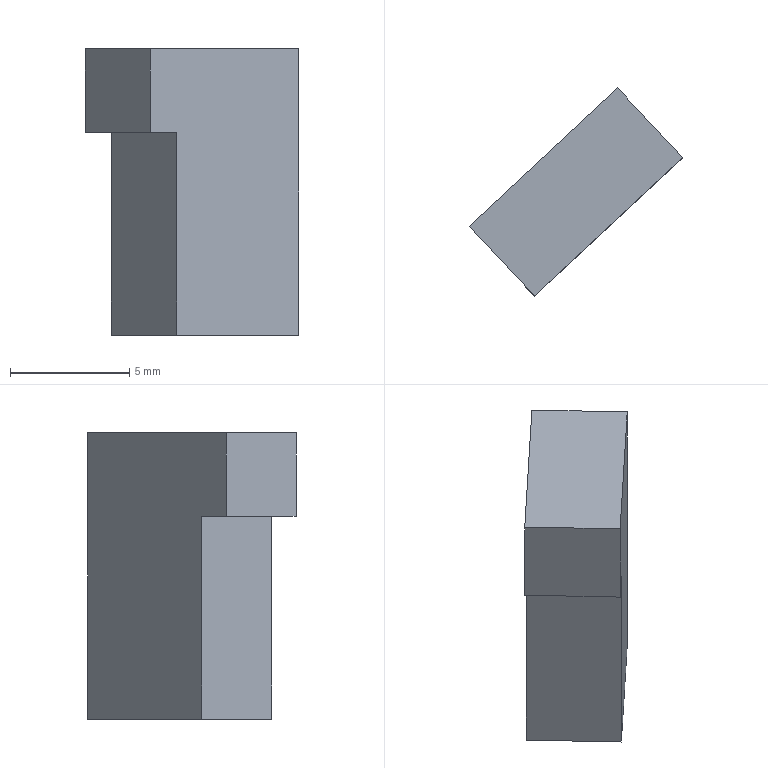Part | STEP file | gslz 2016.10.28-13_id946_x_t | 1 solid | 8 faces | box 8.945 x 8.722 x 12 mm | volume 357 mm3 | plane 8
STEP:
#1=CARTESIAN_POINT('',(0.,0.,0.));
#2=DIRECTION('',(0.,0.,1.));
#3=DIRECTION('',(1.,0.,0.));
#4=AXIS2_PLACEMENT_3D('',#1,#2,#3);
#5=CARTESIAN_POINT('',(-472.551,139.078,1.25));
#6=VERTEX_POINT('',#5);
#7=CARTESIAN_POINT('',(-467.431,143.852,1.25));
#8=VERTEX_POINT('',#7);
#9=CARTESIAN_POINT('',(-472.551,139.078,1.25));
#10=DIRECTION('',(0.7314,0.682,0.));
#11=VECTOR('',#10,1.);
#12=LINE('',#9,#11);
#13=CARTESIAN_POINT('',(-469.961,152.43,1.25));
#14=DIRECTION('',(0.,0.,-1.));
#15=DIRECTION('',(0.7314,0.682,0.));
#16=AXIS2_PLACEMENT_3D('',#13,#14,#15);
#17=PLANE('',#16);
#18=CARTESIAN_POINT('',(-11.,7.999));
#19=DIRECTION('',(1.,0.));
#20=VECTOR('',#19,1.);
#21=LINE('',#18,#20);
#22=(GEOMETRIC_REPRESENTATION_CONTEXT(2)PARAMETRIC_REPRESENTATION_CONTEXT()REPRESENTATION_CONTEXT('',''));
#23=DEFINITIONAL_REPRESENTATION('',(#21),#22);
#24=PCURVE('',#17,#23);
#25=CARTESIAN_POINT('',(-472.551,139.078,-0.75));
#26=DIRECTION('',(0.682,-0.7314,0.));
#27=DIRECTION('',(0.,0.,-1.));
#28=AXIS2_PLACEMENT_3D('',#25,#26,#27);
#29=PLANE('',#28);
#30=CARTESIAN_POINT('',(-2.,0.));
#31=DIRECTION('',(0.,1.));
#32=VECTOR('',#31,1.);
#33=LINE('',#30,#32);
#34=(GEOMETRIC_REPRESENTATION_CONTEXT(2)PARAMETRIC_REPRESENTATION_CONTEXT()REPRESENTATION_CONTEXT('',''));
#35=DEFINITIONAL_REPRESENTATION('',(#33),#34);
#36=PCURVE('',#29,#35);
#37=SURFACE_CURVE('',#12,(#24,#36),.PCURVE_S1.);
#38=EDGE_CURVE('',#6,#8,#37,.T.);
#39=ORIENTED_EDGE('',*,*,#38,.T.);
#40=CARTESIAN_POINT('',(-464.703,140.927,1.25));
#41=VERTEX_POINT('',#40);
#42=CARTESIAN_POINT('',(-467.431,143.852,1.25));
#43=DIRECTION('',(0.682,-0.7314,0.));
#44=VECTOR('',#43,1.);
#45=LINE('',#42,#44);
#46=CARTESIAN_POINT('',(-4.,7.999));
#47=DIRECTION('',(0.,1.));
#48=VECTOR('',#47,1.);
#49=LINE('',#46,#48);
#50=(GEOMETRIC_REPRESENTATION_CONTEXT(2)PARAMETRIC_REPRESENTATION_CONTEXT()REPRESENTATION_CONTEXT('',''));
#51=DEFINITIONAL_REPRESENTATION('',(#49),#50);
#52=PCURVE('',#17,#51);
#53=CARTESIAN_POINT('',(-467.431,143.852,-0.75));
#54=DIRECTION('',(-0.7314,-0.682,0.));
#55=DIRECTION('',(0.,0.,-1.));
#56=AXIS2_PLACEMENT_3D('',#53,#54,#55);
#57=PLANE('',#56);
#58=CARTESIAN_POINT('',(-2.,0.));
#59=DIRECTION('',(0.,1.));
#60=VECTOR('',#59,1.);
#61=LINE('',#58,#60);
#62=(GEOMETRIC_REPRESENTATION_CONTEXT(2)PARAMETRIC_REPRESENTATION_CONTEXT()REPRESENTATION_CONTEXT('',''));
#63=DEFINITIONAL_REPRESENTATION('',(#61),#62);
#64=PCURVE('',#57,#63);
#65=SURFACE_CURVE('',#45,(#52,#64),.PCURVE_S1.);
#66=EDGE_CURVE('',#8,#41,#65,.T.);
#67=ORIENTED_EDGE('',*,*,#66,.T.);
#68=CARTESIAN_POINT('',(-469.823,136.153,1.25));
#69=VERTEX_POINT('',#68);
#70=CARTESIAN_POINT('',(-464.703,140.927,1.25));
#71=DIRECTION('',(-0.7314,-0.682,0.));
#72=VECTOR('',#71,1.);
#73=LINE('',#70,#72);
#74=CARTESIAN_POINT('',(-4.,11.999));
#75=DIRECTION('',(-1.,0.));
#76=VECTOR('',#75,1.);
#77=LINE('',#74,#76);
#78=(GEOMETRIC_REPRESENTATION_CONTEXT(2)PARAMETRIC_REPRESENTATION_CONTEXT()REPRESENTATION_CONTEXT('',''));
#79=DEFINITIONAL_REPRESENTATION('',(#77),#78);
#80=PCURVE('',#17,#79);
#81=CARTESIAN_POINT('',(-464.703,140.927,-0.75));
#82=DIRECTION('',(-0.682,0.7314,0.));
#83=DIRECTION('',(0.,0.,1.));
#84=AXIS2_PLACEMENT_3D('',#81,#82,#83);
#85=PLANE('',#84);
#86=CARTESIAN_POINT('',(2.,0.));
#87=DIRECTION('',(0.,-1.));
#88=VECTOR('',#87,1.);
#89=LINE('',#86,#88);
#90=(GEOMETRIC_REPRESENTATION_CONTEXT(2)PARAMETRIC_REPRESENTATION_CONTEXT()REPRESENTATION_CONTEXT('',''));
#91=DEFINITIONAL_REPRESENTATION('',(#89),#90);
#92=PCURVE('',#85,#91);
#93=SURFACE_CURVE('',#73,(#80,#92),.PCURVE_S1.);
#94=EDGE_CURVE('',#41,#69,#93,.T.);
#95=ORIENTED_EDGE('',*,*,#94,.T.);
#96=CARTESIAN_POINT('',(-469.823,136.153,1.25));
#97=DIRECTION('',(-0.682,0.7314,0.));
#98=VECTOR('',#97,1.);
#99=LINE('',#96,#98);
#100=CARTESIAN_POINT('',(-11.,11.999));
#101=DIRECTION('',(0.,-1.));
#102=VECTOR('',#101,1.);
#103=LINE('',#100,#102);
#104=(GEOMETRIC_REPRESENTATION_CONTEXT(2)PARAMETRIC_REPRESENTATION_CONTEXT()REPRESENTATION_CONTEXT('',''));
#105=DEFINITIONAL_REPRESENTATION('',(#103),#104);
#106=PCURVE('',#17,#105);
#107=CARTESIAN_POINT('',(-469.823,136.153,-0.75));
#108=DIRECTION('',(0.7314,0.682,0.));
#109=DIRECTION('',(0.,0.,1.));
#110=AXIS2_PLACEMENT_3D('',#107,#108,#109);
#111=PLANE('',#110);
#112=CARTESIAN_POINT('',(2.,0.));
#113=DIRECTION('',(0.,-1.));
#114=VECTOR('',#113,1.);
#115=LINE('',#112,#114);
#116=(GEOMETRIC_REPRESENTATION_CONTEXT(2)PARAMETRIC_REPRESENTATION_CONTEXT()REPRESENTATION_CONTEXT('',''));
#117=DEFINITIONAL_REPRESENTATION('',(#115),#116);
#118=PCURVE('',#111,#117);
#119=SURFACE_CURVE('',#99,(#106,#118),.PCURVE_S1.);
#120=EDGE_CURVE('',#69,#6,#119,.T.);
#121=ORIENTED_EDGE('',*,*,#120,.T.);
#122=EDGE_LOOP('',(#39,#67,#95,#121));
#123=FACE_BOUND('',#122,.T.);
#124=ADVANCED_FACE('',(#123),#17,.T.);
#125=CARTESIAN_POINT('',(-473.648,138.055,13.25));
#126=VERTEX_POINT('',#125);
#127=CARTESIAN_POINT('',(-467.431,143.852,13.25));
#128=VERTEX_POINT('',#127);
#129=CARTESIAN_POINT('',(-472.551,139.078,13.25));
#130=DIRECTION('',(0.7314,0.682,0.));
#131=VECTOR('',#130,1.);
#132=LINE('',#129,#131);
#133=CARTESIAN_POINT('',(-14.,0.));
#134=DIRECTION('',(0.,1.));
#135=VECTOR('',#134,1.);
#136=LINE('',#133,#135);
#137=(GEOMETRIC_REPRESENTATION_CONTEXT(2)PARAMETRIC_REPRESENTATION_CONTEXT()REPRESENTATION_CONTEXT('',''));
#138=DEFINITIONAL_REPRESENTATION('',(#136),#137);
#139=PCURVE('',#29,#138);
#140=CARTESIAN_POINT('',(-469.961,152.43,13.25));
#141=DIRECTION('',(0.,0.,-1.));
#142=DIRECTION('',(0.7314,0.682,0.));
#143=AXIS2_PLACEMENT_3D('',#140,#141,#142);
#144=PLANE('',#143);
#145=CARTESIAN_POINT('',(-11.,7.999));
#146=DIRECTION('',(1.,0.));
#147=VECTOR('',#146,1.);
#148=LINE('',#145,#147);
#149=(GEOMETRIC_REPRESENTATION_CONTEXT(2)PARAMETRIC_REPRESENTATION_CONTEXT()REPRESENTATION_CONTEXT('',''));
#150=DEFINITIONAL_REPRESENTATION('',(#148),#149);
#151=PCURVE('',#144,#150);
#152=SURFACE_CURVE('',#132,(#139,#151),.PCURVE_S1.);
#153=EDGE_CURVE('',#126,#128,#152,.T.);
#154=ORIENTED_EDGE('',*,*,#153,.T.);
#155=CARTESIAN_POINT('',(-467.431,143.852,-0.75));
#156=DIRECTION('',(0.,0.,1.));
#157=VECTOR('',#156,1.);
#158=LINE('',#155,#157);
#159=CARTESIAN_POINT('',(0.,7.));
#160=DIRECTION('',(-1.,0.));
#161=VECTOR('',#160,1.);
#162=LINE('',#159,#161);
#163=(GEOMETRIC_REPRESENTATION_CONTEXT(2)PARAMETRIC_REPRESENTATION_CONTEXT()REPRESENTATION_CONTEXT('',''));
#164=DEFINITIONAL_REPRESENTATION('',(#162),#163);
#165=PCURVE('',#29,#164);
#166=CARTESIAN_POINT('',(0.,0.));
#167=DIRECTION('',(-1.,0.));
#168=VECTOR('',#167,1.);
#169=LINE('',#166,#168);
#170=(GEOMETRIC_REPRESENTATION_CONTEXT(2)PARAMETRIC_REPRESENTATION_CONTEXT()REPRESENTATION_CONTEXT('',''));
#171=DEFINITIONAL_REPRESENTATION('',(#169),#170);
#172=PCURVE('',#57,#171);
#173=SURFACE_CURVE('',#158,(#165,#172),.PCURVE_S1.);
#174=EDGE_CURVE('',#8,#128,#173,.T.);
#175=ORIENTED_EDGE('',*,*,#174,.F.);
#176=ORIENTED_EDGE('',*,*,#38,.F.);
#177=CARTESIAN_POINT('',(-472.551,139.078,9.75));
#178=VERTEX_POINT('',#177);
#179=CARTESIAN_POINT('',(-472.551,139.078,-0.75));
#180=DIRECTION('',(0.,0.,1.));
#181=VECTOR('',#180,1.);
#182=LINE('',#179,#181);
#183=CARTESIAN_POINT('',(0.,0.));
#184=DIRECTION('',(-1.,0.));
#185=VECTOR('',#184,1.);
#186=LINE('',#183,#185);
#187=(GEOMETRIC_REPRESENTATION_CONTEXT(2)PARAMETRIC_REPRESENTATION_CONTEXT()REPRESENTATION_CONTEXT('',''));
#188=DEFINITIONAL_REPRESENTATION('',(#186),#187);
#189=PCURVE('',#29,#188);
#190=CARTESIAN_POINT('',(0.,-4.));
#191=DIRECTION('',(1.,0.));
#192=VECTOR('',#191,1.);
#193=LINE('',#190,#192);
#194=(GEOMETRIC_REPRESENTATION_CONTEXT(2)PARAMETRIC_REPRESENTATION_CONTEXT()REPRESENTATION_CONTEXT('',''));
#195=DEFINITIONAL_REPRESENTATION('',(#193),#194);
#196=PCURVE('',#111,#195);
#197=SURFACE_CURVE('',#182,(#189,#196),.PCURVE_S1.);
#198=EDGE_CURVE('',#6,#178,#197,.T.);
#199=ORIENTED_EDGE('',*,*,#198,.T.);
#200=CARTESIAN_POINT('',(-473.648,138.055,9.75));
#201=VERTEX_POINT('',#200);
#202=CARTESIAN_POINT('',(-473.648,138.055,9.75));
#203=DIRECTION('',(0.7314,0.682,0.));
#204=VECTOR('',#203,1.);
#205=LINE('',#202,#204);
#206=CARTESIAN_POINT('',(-10.5,-1.5));
#207=DIRECTION('',(0.,1.));
#208=VECTOR('',#207,1.);
#209=LINE('',#206,#208);
#210=(GEOMETRIC_REPRESENTATION_CONTEXT(2)PARAMETRIC_REPRESENTATION_CONTEXT()REPRESENTATION_CONTEXT('',''));
#211=DEFINITIONAL_REPRESENTATION('',(#209),#210);
#212=PCURVE('',#29,#211);
#213=CARTESIAN_POINT('',(-470.92,135.13,9.75));
#214=DIRECTION('',(0.,0.,-1.));
#215=DIRECTION('',(0.7314,0.682,0.));
#216=AXIS2_PLACEMENT_3D('',#213,#214,#215);
#217=PLANE('',#216);
#218=CARTESIAN_POINT('',(0.,-4.));
#219=DIRECTION('',(1.,0.));
#220=VECTOR('',#219,1.);
#221=LINE('',#218,#220);
#222=(GEOMETRIC_REPRESENTATION_CONTEXT(2)PARAMETRIC_REPRESENTATION_CONTEXT()REPRESENTATION_CONTEXT('',''));
#223=DEFINITIONAL_REPRESENTATION('',(#221),#222);
#224=PCURVE('',#217,#223);
#225=SURFACE_CURVE('',#205,(#212,#224),.PCURVE_S1.);
#226=EDGE_CURVE('',#201,#178,#225,.T.);
#227=ORIENTED_EDGE('',*,*,#226,.F.);
#228=CARTESIAN_POINT('',(-473.648,138.055,13.25));
#229=DIRECTION('',(0.,0.,-1.));
#230=VECTOR('',#229,1.);
#231=LINE('',#228,#230);
#232=CARTESIAN_POINT('',(-14.,-1.5));
#233=DIRECTION('',(1.,0.));
#234=VECTOR('',#233,1.);
#235=LINE('',#232,#234);
#236=(GEOMETRIC_REPRESENTATION_CONTEXT(2)PARAMETRIC_REPRESENTATION_CONTEXT()REPRESENTATION_CONTEXT('',''));
#237=DEFINITIONAL_REPRESENTATION('',(#235),#236);
#238=PCURVE('',#29,#237);
#239=CARTESIAN_POINT('',(-470.92,135.13,13.25));
#240=DIRECTION('',(-0.7314,-0.682,0.));
#241=DIRECTION('',(-0.682,0.7314,0.));
#242=AXIS2_PLACEMENT_3D('',#239,#240,#241);
#243=PLANE('',#242);
#244=CARTESIAN_POINT('',(4.,0.));
#245=DIRECTION('',(0.,1.));
#246=VECTOR('',#245,1.);
#247=LINE('',#244,#246);
#248=(GEOMETRIC_REPRESENTATION_CONTEXT(2)PARAMETRIC_REPRESENTATION_CONTEXT()REPRESENTATION_CONTEXT('',''));
#249=DEFINITIONAL_REPRESENTATION('',(#247),#248);
#250=PCURVE('',#243,#249);
#251=SURFACE_CURVE('',#231,(#238,#250),.PCURVE_S1.);
#252=EDGE_CURVE('',#126,#201,#251,.T.);
#253=ORIENTED_EDGE('',*,*,#252,.F.);
#254=EDGE_LOOP('',(#154,#175,#176,#199,#227,#253));
#255=FACE_BOUND('',#254,.T.);
#256=ADVANCED_FACE('',(#255),#29,.F.);
#257=CARTESIAN_POINT('',(-464.703,140.927,13.25));
#258=VERTEX_POINT('',#257);
#259=CARTESIAN_POINT('',(-467.431,143.852,13.25));
#260=DIRECTION('',(0.682,-0.7314,0.));
#261=VECTOR('',#260,1.);
#262=LINE('',#259,#261);
#263=CARTESIAN_POINT('',(-14.,0.));
#264=DIRECTION('',(0.,1.));
#265=VECTOR('',#264,1.);
#266=LINE('',#263,#265);
#267=(GEOMETRIC_REPRESENTATION_CONTEXT(2)PARAMETRIC_REPRESENTATION_CONTEXT()REPRESENTATION_CONTEXT('',''));
#268=DEFINITIONAL_REPRESENTATION('',(#266),#267);
#269=PCURVE('',#57,#268);
#270=CARTESIAN_POINT('',(-4.,7.999));
#271=DIRECTION('',(0.,1.));
#272=VECTOR('',#271,1.);
#273=LINE('',#270,#272);
#274=(GEOMETRIC_REPRESENTATION_CONTEXT(2)PARAMETRIC_REPRESENTATION_CONTEXT()REPRESENTATION_CONTEXT('',''));
#275=DEFINITIONAL_REPRESENTATION('',(#273),#274);
#276=PCURVE('',#144,#275);
#277=SURFACE_CURVE('',#262,(#269,#276),.PCURVE_S1.);
#278=EDGE_CURVE('',#128,#258,#277,.T.);
#279=ORIENTED_EDGE('',*,*,#278,.T.);
#280=CARTESIAN_POINT('',(-464.703,140.927,-0.75));
#281=DIRECTION('',(0.,0.,1.));
#282=VECTOR('',#281,1.);
#283=LINE('',#280,#282);
#284=CARTESIAN_POINT('',(0.,4.));
#285=DIRECTION('',(-1.,0.));
#286=VECTOR('',#285,1.);
#287=LINE('',#284,#286);
#288=(GEOMETRIC_REPRESENTATION_CONTEXT(2)PARAMETRIC_REPRESENTATION_CONTEXT()REPRESENTATION_CONTEXT('',''));
#289=DEFINITIONAL_REPRESENTATION('',(#287),#288);
#290=PCURVE('',#57,#289);
#291=CARTESIAN_POINT('',(0.,0.));
#292=DIRECTION('',(1.,0.));
#293=VECTOR('',#292,1.);
#294=LINE('',#291,#293);
#295=(GEOMETRIC_REPRESENTATION_CONTEXT(2)PARAMETRIC_REPRESENTATION_CONTEXT()REPRESENTATION_CONTEXT('',''));
#296=DEFINITIONAL_REPRESENTATION('',(#294),#295);
#297=PCURVE('',#85,#296);
#298=SURFACE_CURVE('',#283,(#290,#297),.PCURVE_S1.);
#299=EDGE_CURVE('',#41,#258,#298,.T.);
#300=ORIENTED_EDGE('',*,*,#299,.F.);
#301=ORIENTED_EDGE('',*,*,#66,.F.);
#302=ORIENTED_EDGE('',*,*,#174,.T.);
#303=EDGE_LOOP('',(#279,#300,#301,#302));
#304=FACE_BOUND('',#303,.T.);
#305=ADVANCED_FACE('',(#304),#57,.F.);
#306=CARTESIAN_POINT('',(-470.92,135.13,13.25));
#307=VERTEX_POINT('',#306);
#308=CARTESIAN_POINT('',(-464.703,140.927,13.25));
#309=DIRECTION('',(-0.7314,-0.682,0.));
#310=VECTOR('',#309,1.);
#311=LINE('',#308,#310);
#312=CARTESIAN_POINT('',(14.,0.));
#313=DIRECTION('',(0.,-1.));
#314=VECTOR('',#313,1.);
#315=LINE('',#312,#314);
#316=(GEOMETRIC_REPRESENTATION_CONTEXT(2)PARAMETRIC_REPRESENTATION_CONTEXT()REPRESENTATION_CONTEXT('',''));
#317=DEFINITIONAL_REPRESENTATION('',(#315),#316);
#318=PCURVE('',#85,#317);
#319=CARTESIAN_POINT('',(-4.,11.999));
#320=DIRECTION('',(-1.,0.));
#321=VECTOR('',#320,1.);
#322=LINE('',#319,#321);
#323=(GEOMETRIC_REPRESENTATION_CONTEXT(2)PARAMETRIC_REPRESENTATION_CONTEXT()REPRESENTATION_CONTEXT('',''));
#324=DEFINITIONAL_REPRESENTATION('',(#322),#323);
#325=PCURVE('',#144,#324);
#326=SURFACE_CURVE('',#311,(#318,#325),.PCURVE_S1.);
#327=EDGE_CURVE('',#258,#307,#326,.T.);
#328=ORIENTED_EDGE('',*,*,#327,.T.);
#329=CARTESIAN_POINT('',(-470.92,135.13,9.75));
#330=VERTEX_POINT('',#329);
#331=CARTESIAN_POINT('',(-470.92,135.13,13.25));
#332=DIRECTION('',(0.,0.,-1.));
#333=VECTOR('',#332,1.);
#334=LINE('',#331,#333);
#335=CARTESIAN_POINT('',(14.,-8.5));
#336=DIRECTION('',(-1.,0.));
#337=VECTOR('',#336,1.);
#338=LINE('',#335,#337);
#339=(GEOMETRIC_REPRESENTATION_CONTEXT(2)PARAMETRIC_REPRESENTATION_CONTEXT()REPRESENTATION_CONTEXT('',''));
#340=DEFINITIONAL_REPRESENTATION('',(#338),#339);
#341=PCURVE('',#85,#340);
#342=CARTESIAN_POINT('',(0.,0.));
#343=DIRECTION('',(0.,1.));
#344=VECTOR('',#343,1.);
#345=LINE('',#342,#344);
#346=(GEOMETRIC_REPRESENTATION_CONTEXT(2)PARAMETRIC_REPRESENTATION_CONTEXT()REPRESENTATION_CONTEXT('',''));
#347=DEFINITIONAL_REPRESENTATION('',(#345),#346);
#348=PCURVE('',#243,#347);
#349=SURFACE_CURVE('',#334,(#341,#348),.PCURVE_S1.);
#350=EDGE_CURVE('',#307,#330,#349,.T.);
#351=ORIENTED_EDGE('',*,*,#350,.T.);
#352=CARTESIAN_POINT('',(-469.823,136.153,9.75));
#353=VERTEX_POINT('',#352);
#354=CARTESIAN_POINT('',(-470.92,135.13,9.75));
#355=DIRECTION('',(0.7314,0.682,0.));
#356=VECTOR('',#355,1.);
#357=LINE('',#354,#356);
#358=CARTESIAN_POINT('',(10.5,-8.5));
#359=DIRECTION('',(0.,1.));
#360=VECTOR('',#359,1.);
#361=LINE('',#358,#360);
#362=(GEOMETRIC_REPRESENTATION_CONTEXT(2)PARAMETRIC_REPRESENTATION_CONTEXT()REPRESENTATION_CONTEXT('',''));
#363=DEFINITIONAL_REPRESENTATION('',(#361),#362);
#364=PCURVE('',#85,#363);
#365=CARTESIAN_POINT('',(0.,0.));
#366=DIRECTION('',(1.,0.));
#367=VECTOR('',#366,1.);
#368=LINE('',#365,#367);
#369=(GEOMETRIC_REPRESENTATION_CONTEXT(2)PARAMETRIC_REPRESENTATION_CONTEXT()REPRESENTATION_CONTEXT('',''));
#370=DEFINITIONAL_REPRESENTATION('',(#368),#369);
#371=PCURVE('',#217,#370);
#372=SURFACE_CURVE('',#357,(#364,#371),.PCURVE_S1.);
#373=EDGE_CURVE('',#330,#353,#372,.T.);
#374=ORIENTED_EDGE('',*,*,#373,.T.);
#375=CARTESIAN_POINT('',(-469.823,136.153,-0.75));
#376=DIRECTION('',(0.,0.,1.));
#377=VECTOR('',#376,1.);
#378=LINE('',#375,#377);
#379=CARTESIAN_POINT('',(0.,-7.));
#380=DIRECTION('',(1.,0.));
#381=VECTOR('',#380,1.);
#382=LINE('',#379,#381);
#383=(GEOMETRIC_REPRESENTATION_CONTEXT(2)PARAMETRIC_REPRESENTATION_CONTEXT()REPRESENTATION_CONTEXT('',''));
#384=DEFINITIONAL_REPRESENTATION('',(#382),#383);
#385=PCURVE('',#85,#384);
#386=CARTESIAN_POINT('',(0.,0.));
#387=DIRECTION('',(1.,0.));
#388=VECTOR('',#387,1.);
#389=LINE('',#386,#388);
#390=(GEOMETRIC_REPRESENTATION_CONTEXT(2)PARAMETRIC_REPRESENTATION_CONTEXT()REPRESENTATION_CONTEXT('',''));
#391=DEFINITIONAL_REPRESENTATION('',(#389),#390);
#392=PCURVE('',#111,#391);
#393=SURFACE_CURVE('',#378,(#385,#392),.PCURVE_S1.);
#394=EDGE_CURVE('',#69,#353,#393,.T.);
#395=ORIENTED_EDGE('',*,*,#394,.F.);
#396=ORIENTED_EDGE('',*,*,#94,.F.);
#397=ORIENTED_EDGE('',*,*,#299,.T.);
#398=EDGE_LOOP('',(#328,#351,#374,#395,#396,#397));
#399=FACE_BOUND('',#398,.T.);
#400=ADVANCED_FACE('',(#399),#85,.F.);
#401=ORIENTED_EDGE('',*,*,#394,.T.);
#402=CARTESIAN_POINT('',(-469.823,136.153,9.75));
#403=DIRECTION('',(-0.682,0.7314,0.));
#404=VECTOR('',#403,1.);
#405=LINE('',#402,#404);
#406=CARTESIAN_POINT('',(10.5,0.));
#407=DIRECTION('',(0.,-1.));
#408=VECTOR('',#407,1.);
#409=LINE('',#406,#408);
#410=(GEOMETRIC_REPRESENTATION_CONTEXT(2)PARAMETRIC_REPRESENTATION_CONTEXT()REPRESENTATION_CONTEXT('',''));
#411=DEFINITIONAL_REPRESENTATION('',(#409),#410);
#412=PCURVE('',#111,#411);
#413=CARTESIAN_POINT('',(1.5,0.));
#414=DIRECTION('',(0.,-1.));
#415=VECTOR('',#414,1.);
#416=LINE('',#413,#415);
#417=(GEOMETRIC_REPRESENTATION_CONTEXT(2)PARAMETRIC_REPRESENTATION_CONTEXT()REPRESENTATION_CONTEXT('',''));
#418=DEFINITIONAL_REPRESENTATION('',(#416),#417);
#419=PCURVE('',#217,#418);
#420=SURFACE_CURVE('',#405,(#412,#419),.PCURVE_S1.);
#421=EDGE_CURVE('',#353,#178,#420,.T.);
#422=ORIENTED_EDGE('',*,*,#421,.T.);
#423=ORIENTED_EDGE('',*,*,#198,.F.);
#424=ORIENTED_EDGE('',*,*,#120,.F.);
#425=EDGE_LOOP('',(#401,#422,#423,#424));
#426=FACE_BOUND('',#425,.T.);
#427=ADVANCED_FACE('',(#426),#111,.F.);
#428=ORIENTED_EDGE('',*,*,#153,.F.);
#429=CARTESIAN_POINT('',(-470.92,135.13,13.25));
#430=DIRECTION('',(-0.682,0.7314,0.));
#431=VECTOR('',#430,1.);
#432=LINE('',#429,#431);
#433=CARTESIAN_POINT('',(-12.5,11.999));
#434=DIRECTION('',(0.,-1.));
#435=VECTOR('',#434,1.);
#436=LINE('',#433,#435);
#437=(GEOMETRIC_REPRESENTATION_CONTEXT(2)PARAMETRIC_REPRESENTATION_CONTEXT()REPRESENTATION_CONTEXT('',''));
#438=DEFINITIONAL_REPRESENTATION('',(#436),#437);
#439=PCURVE('',#144,#438);
#440=CARTESIAN_POINT('',(0.,0.));
#441=DIRECTION('',(1.,0.));
#442=VECTOR('',#441,1.);
#443=LINE('',#440,#442);
#444=(GEOMETRIC_REPRESENTATION_CONTEXT(2)PARAMETRIC_REPRESENTATION_CONTEXT()REPRESENTATION_CONTEXT('',''));
#445=DEFINITIONAL_REPRESENTATION('',(#443),#444);
#446=PCURVE('',#243,#445);
#447=SURFACE_CURVE('',#432,(#439,#446),.PCURVE_S1.);
#448=EDGE_CURVE('',#307,#126,#447,.T.);
#449=ORIENTED_EDGE('',*,*,#448,.F.);
#450=ORIENTED_EDGE('',*,*,#327,.F.);
#451=ORIENTED_EDGE('',*,*,#278,.F.);
#452=EDGE_LOOP('',(#428,#449,#450,#451));
#453=FACE_BOUND('',#452,.T.);
#454=ADVANCED_FACE('',(#453),#144,.F.);
#455=ORIENTED_EDGE('',*,*,#350,.F.);
#456=ORIENTED_EDGE('',*,*,#448,.T.);
#457=ORIENTED_EDGE('',*,*,#252,.T.);
#458=CARTESIAN_POINT('',(-470.92,135.13,9.75));
#459=DIRECTION('',(-0.682,0.7314,0.));
#460=VECTOR('',#459,1.);
#461=LINE('',#458,#460);
#462=CARTESIAN_POINT('',(0.,3.5));
#463=DIRECTION('',(1.,0.));
#464=VECTOR('',#463,1.);
#465=LINE('',#462,#464);
#466=(GEOMETRIC_REPRESENTATION_CONTEXT(2)PARAMETRIC_REPRESENTATION_CONTEXT()REPRESENTATION_CONTEXT('',''));
#467=DEFINITIONAL_REPRESENTATION('',(#465),#466);
#468=PCURVE('',#243,#467);
#469=CARTESIAN_POINT('',(0.,0.));
#470=DIRECTION('',(0.,-1.));
#471=VECTOR('',#470,1.);
#472=LINE('',#469,#471);
#473=(GEOMETRIC_REPRESENTATION_CONTEXT(2)PARAMETRIC_REPRESENTATION_CONTEXT()REPRESENTATION_CONTEXT('',''));
#474=DEFINITIONAL_REPRESENTATION('',(#472),#473);
#475=PCURVE('',#217,#474);
#476=SURFACE_CURVE('',#461,(#468,#475),.PCURVE_S1.);
#477=EDGE_CURVE('',#330,#201,#476,.T.);
#478=ORIENTED_EDGE('',*,*,#477,.F.);
#479=EDGE_LOOP('',(#455,#456,#457,#478));
#480=FACE_BOUND('',#479,.T.);
#481=ADVANCED_FACE('',(#480),#243,.T.);
#482=ORIENTED_EDGE('',*,*,#421,.F.);
#483=ORIENTED_EDGE('',*,*,#373,.F.);
#484=ORIENTED_EDGE('',*,*,#477,.T.);
#485=ORIENTED_EDGE('',*,*,#226,.T.);
#486=EDGE_LOOP('',(#482,#483,#484,#485));
#487=FACE_BOUND('',#486,.T.);
#488=ADVANCED_FACE('',(#487),#217,.T.);
#489=CLOSED_SHELL('',(#124,#256,#305,#400,#427,#454,#481,#488));
#490=MANIFOLD_SOLID_BREP('',#489);
#491=(LENGTH_UNIT()NAMED_UNIT(*)SI_UNIT(.MILLI.,.METRE.));
#492=UNCERTAINTY_MEASURE_WITH_UNIT(LENGTH_MEASURE(0.0000001),#491,'','');
#493=(NAMED_UNIT(*)PLANE_ANGLE_UNIT()SI_UNIT($,.RADIAN.));
#494=(NAMED_UNIT(*)SI_UNIT($,.STERADIAN.)SOLID_ANGLE_UNIT());
#495=(GEOMETRIC_REPRESENTATION_CONTEXT(3)GLOBAL_UNCERTAINTY_ASSIGNED_CONTEXT((#492))GLOBAL_UNIT_ASSIGNED_CONTEXT((#491,#493,#494))REPRESENTATION_CONTEXT('',''));
#496=ADVANCED_BREP_SHAPE_REPRESENTATION('',(#4,#490),#495);